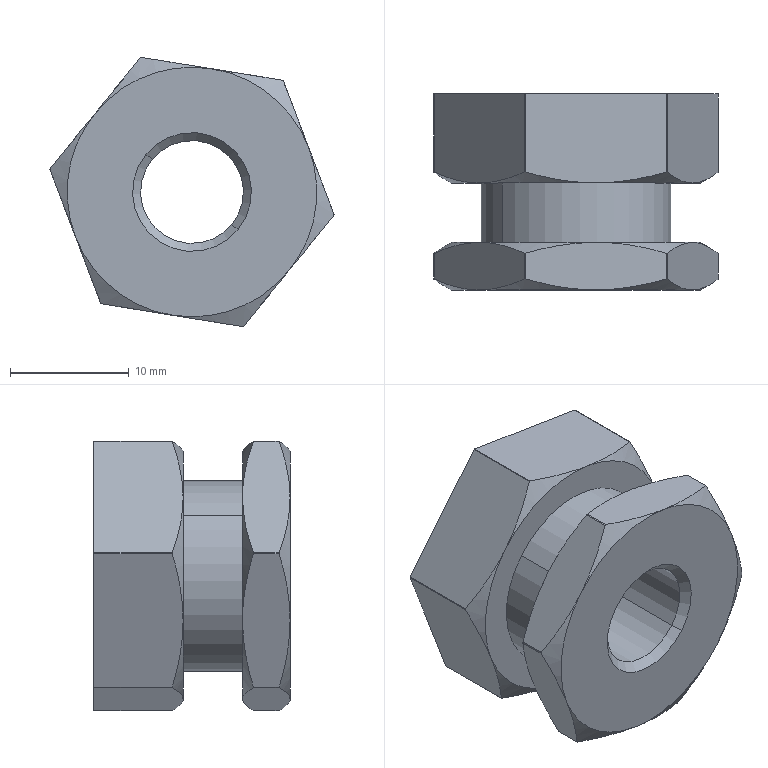Part | NX | features WHC31-M10-1_25-L8.SLDPRT 2 | 1 solid | 52 faces | box 23.903 x 16.5 x 22.65 mm | volume 4391 mm3 | cone 20 | cylinder 16 | plane 16 | commonest cylinder face diameters 24.2 x12 8.647 x2 16 x2